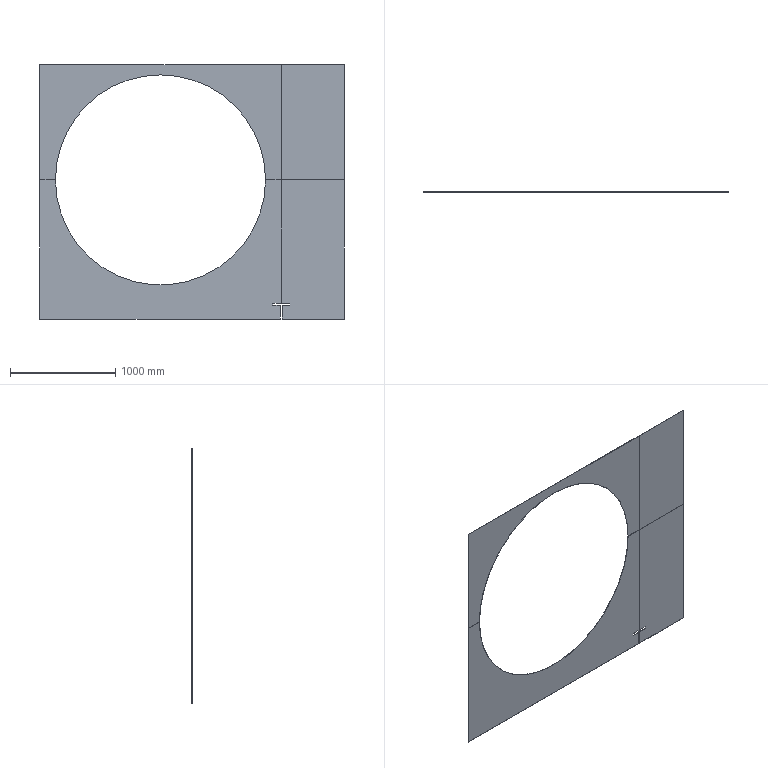Part | STEP file | Bracket花纹Plate 9 | 4 solids | 39 faces | box 2900 x 3 x 2420 mm | volume 11613706 mm3 | plane 34 | cylinder 5 | commonest cylinder face diameters 2000 x3 6 x2